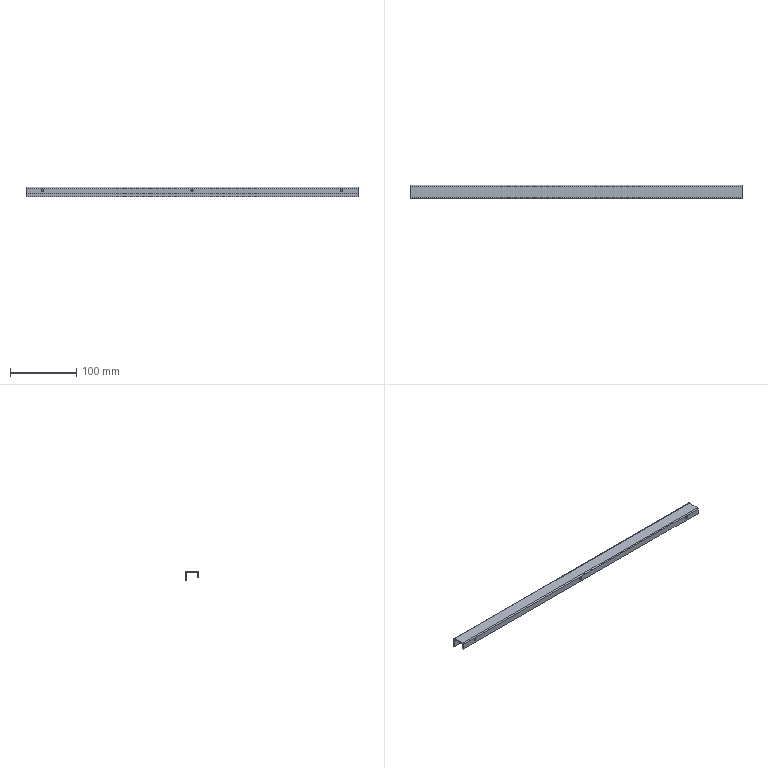Part | STEP file | HESS-408-70-15W-D-10-edge strip 2 | 1 solid | 20 faces | box 500 x 20 x 15 mm | volume 30917 mm3 | cylinder 10 | plane 10 | commonest cylinder face diameters 3.2 x8 0.2 x2